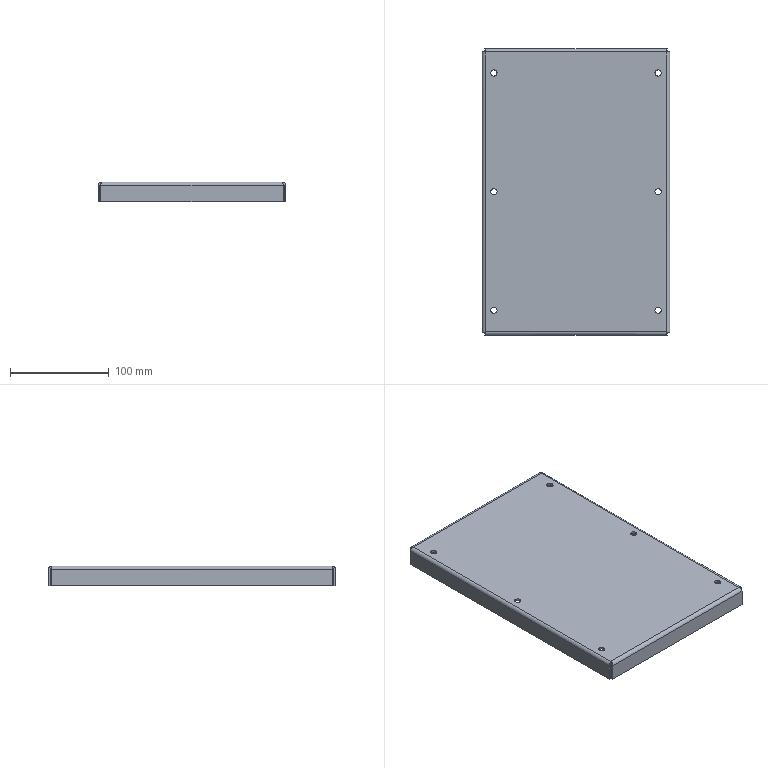Part | STEP file | Motor side cover plate SGN-2-31-02 | 1 solid | 50 faces | box 190 x 290 x 20 mm | volume 141514 mm3 | plane 22 | cylinder 20 | spline 8 | commonest cylinder face diameters 6.3 x12 3 x4 7 x4